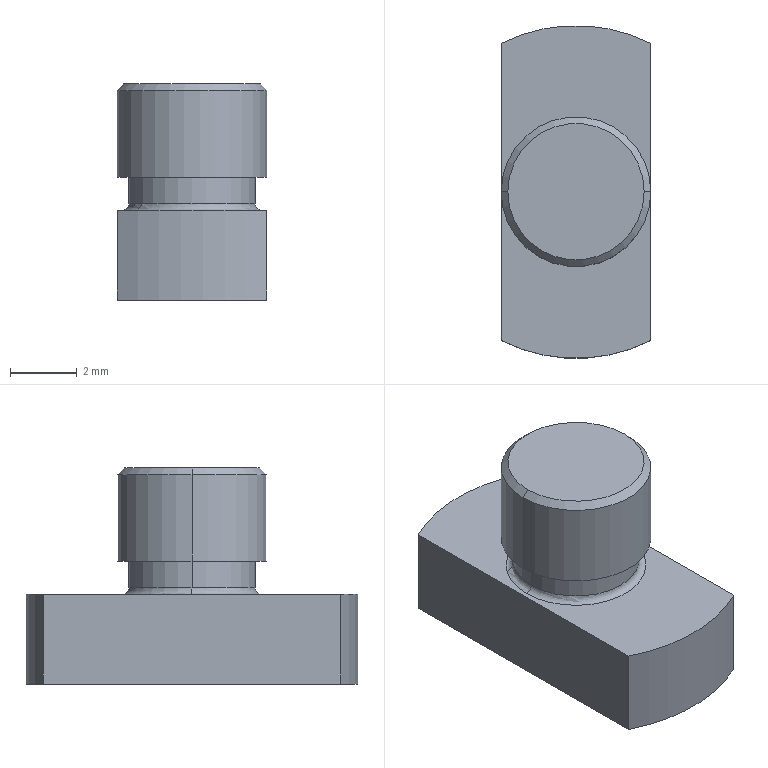Part | SolidWorks | features BaseBody 1 | 1 solid | 16 faces | box 4.5 x 10 x 6.5 mm | volume 172.969 mm3 | cylinder 6 | plane 6 | torus 2 | cone 2 | commonest cylinder face diameters 3.8 x2 4.5 x2 10 x2
STEP:
#1=CARTESIAN_POINT('',(76.4,38.,-17.3));
#2=VERTEX_POINT('',#1);
#3=CARTESIAN_POINT('',(72.6,38.,-17.3));
#4=VERTEX_POINT('',#3);
#5=CARTESIAN_POINT('',(74.5,38.,-17.3));
#6=DIRECTION('',(0.,0.,1.));
#7=DIRECTION('',(-1.,0.,0.));
#8=AXIS2_PLACEMENT_3D('',#5,#6,#7);
#9=CIRCLE('',#8,1.9);
#10=EDGE_CURVE('',#2,#4,#9,.T.);
#11=ORIENTED_EDGE('',*,*,#10,.F.);
#12=CARTESIAN_POINT('',(76.6,38.,-17.5));
#13=VERTEX_POINT('',#12);
#14=CARTESIAN_POINT('',(76.6,38.,-17.3));
#15=DIRECTION('',(0.,-1.,0.));
#16=DIRECTION('',(1.,0.,0.));
#17=AXIS2_PLACEMENT_3D('',#14,#15,#16);
#18=CIRCLE('',#17,0.2);
#19=EDGE_CURVE('',#2,#13,#18,.T.);
#20=ORIENTED_EDGE('',*,*,#19,.T.);
#21=CARTESIAN_POINT('',(72.4,38.,-17.5));
#22=VERTEX_POINT('',#21);
#23=CARTESIAN_POINT('',(74.5,38.,-17.5));
#24=DIRECTION('',(0.,0.,-1.));
#25=DIRECTION('',(-1.,0.,0.));
#26=AXIS2_PLACEMENT_3D('',#23,#24,#25);
#27=CIRCLE('',#26,2.1);
#28=EDGE_CURVE('',#22,#13,#27,.T.);
#29=ORIENTED_EDGE('',*,*,#28,.F.);
#30=CARTESIAN_POINT('',(72.4,38.,-17.3));
#31=DIRECTION('',(0.,1.,0.));
#32=DIRECTION('',(-1.,0.,0.));
#33=AXIS2_PLACEMENT_3D('',#30,#31,#32);
#34=CIRCLE('',#33,0.2);
#35=EDGE_CURVE('',#4,#22,#34,.T.);
#36=ORIENTED_EDGE('',*,*,#35,.F.);
#37=EDGE_LOOP('',(#11,#20,#29,#36));
#38=FACE_OUTER_BOUND('',#37,.T.);
#39=CARTESIAN_POINT('',(74.5,38.,-17.3));
#40=DIRECTION('',(0.,0.,1.));
#41=DIRECTION('',(-1.,0.,0.));
#42=AXIS2_PLACEMENT_3D('',#39,#40,#41);
#43=TOROIDAL_SURFACE('',#42,2.1,0.2);
#44=ADVANCED_FACE('',(#38),#43,.F.);
#45=CARTESIAN_POINT('',(76.55,38.,-13.7));
#46=VERTEX_POINT('',#45);
#47=CARTESIAN_POINT('',(72.45,38.,-13.7));
#48=VERTEX_POINT('',#47);
#49=CARTESIAN_POINT('',(74.5,38.,-13.7));
#50=DIRECTION('',(0.,0.,-1.));
#51=DIRECTION('',(1.,0.,0.));
#52=AXIS2_PLACEMENT_3D('',#49,#50,#51);
#53=CIRCLE('',#52,2.05);
#54=EDGE_CURVE('',#46,#48,#53,.T.);
#55=ORIENTED_EDGE('',*,*,#54,.T.);
#56=CARTESIAN_POINT('',(72.25,38.,-13.9));
#57=VERTEX_POINT('',#56);
#58=CARTESIAN_POINT('',(72.25,38.,-13.9));
#59=DIRECTION('',(-0.7071,0.,-0.7071));
#60=VECTOR('',#59,1000.);
#61=LINE('',#58,#60);
#62=EDGE_CURVE('',#48,#57,#61,.T.);
#63=ORIENTED_EDGE('',*,*,#62,.T.);
#64=CARTESIAN_POINT('',(76.75,38.,-13.9));
#65=VERTEX_POINT('',#64);
#66=CARTESIAN_POINT('',(74.5,38.,-13.9));
#67=DIRECTION('',(0.,0.,-1.));
#68=DIRECTION('',(1.,0.,0.));
#69=AXIS2_PLACEMENT_3D('',#66,#67,#68);
#70=CIRCLE('',#69,2.25);
#71=EDGE_CURVE('',#65,#57,#70,.T.);
#72=ORIENTED_EDGE('',*,*,#71,.F.);
#73=CARTESIAN_POINT('',(76.75,38.,-13.9));
#74=DIRECTION('',(0.7071,0.,-0.7071));
#75=VECTOR('',#74,1000.);
#76=LINE('',#73,#75);
#77=EDGE_CURVE('',#46,#65,#76,.T.);
#78=ORIENTED_EDGE('',*,*,#77,.F.);
#79=EDGE_LOOP('',(#55,#63,#72,#78));
#80=FACE_OUTER_BOUND('',#79,.T.);
#81=CARTESIAN_POINT('',(74.5,38.,-13.9));
#82=DIRECTION('',(0.,0.,-1.));
#83=DIRECTION('',(1.,0.,0.));
#84=AXIS2_PLACEMENT_3D('',#81,#82,#83);
#85=CONICAL_SURFACE('',#84,2.25,0.7854);
#86=ADVANCED_FACE('',(#80),#85,.T.);
#87=ORIENTED_EDGE('',*,*,#71,.T.);
#88=CARTESIAN_POINT('',(72.25,38.,-16.5));
#89=VERTEX_POINT('',#88);
#90=CARTESIAN_POINT('',(72.25,38.,-20.2));
#91=DIRECTION('',(0.,0.,-1.));
#92=VECTOR('',#91,1000.);
#93=LINE('',#90,#92);
#94=EDGE_CURVE('',#57,#89,#93,.T.);
#95=ORIENTED_EDGE('',*,*,#94,.T.);
#96=CARTESIAN_POINT('',(76.75,38.,-16.5));
#97=VERTEX_POINT('',#96);
#98=CARTESIAN_POINT('',(74.5,38.,-16.5));
#99=DIRECTION('',(0.,0.,-1.));
#100=DIRECTION('',(1.,0.,0.));
#101=AXIS2_PLACEMENT_3D('',#98,#99,#100);
#102=CIRCLE('',#101,2.25);
#103=EDGE_CURVE('',#97,#89,#102,.T.);
#104=ORIENTED_EDGE('',*,*,#103,.F.);
#105=CARTESIAN_POINT('',(76.75,38.,-20.2));
#106=DIRECTION('',(0.,0.,-1.));
#107=VECTOR('',#106,1000.);
#108=LINE('',#105,#107);
#109=EDGE_CURVE('',#65,#97,#108,.T.);
#110=ORIENTED_EDGE('',*,*,#109,.F.);
#111=EDGE_LOOP('',(#87,#95,#104,#110));
#112=FACE_OUTER_BOUND('',#111,.T.);
#113=CARTESIAN_POINT('',(74.5,38.,-20.2));
#114=DIRECTION('',(0.,0.,-1.));
#115=DIRECTION('',(1.,0.,0.));
#116=AXIS2_PLACEMENT_3D('',#113,#114,#115);
#117=CYLINDRICAL_SURFACE('',#116,2.25);
#118=ADVANCED_FACE('',(#112),#117,.T.);
#119=CARTESIAN_POINT('',(76.4,38.,-16.5));
#120=VERTEX_POINT('',#119);
#121=CARTESIAN_POINT('',(72.6,38.,-16.5));
#122=VERTEX_POINT('',#121);
#123=CARTESIAN_POINT('',(74.5,38.,-16.5));
#124=DIRECTION('',(0.,0.,-1.));
#125=DIRECTION('',(1.,0.,0.));
#126=AXIS2_PLACEMENT_3D('',#123,#124,#125);
#127=CIRCLE('',#126,1.9);
#128=EDGE_CURVE('',#120,#122,#127,.T.);
#129=ORIENTED_EDGE('',*,*,#128,.T.);
#130=CARTESIAN_POINT('',(72.6,38.,-20.2));
#131=DIRECTION('',(0.,0.,-1.));
#132=VECTOR('',#131,1000.);
#133=LINE('',#130,#132);
#134=EDGE_CURVE('',#122,#4,#133,.T.);
#135=ORIENTED_EDGE('',*,*,#134,.T.);
#136=CARTESIAN_POINT('',(74.5,38.,-17.3));
#137=DIRECTION('',(0.,0.,1.));
#138=DIRECTION('',(-1.,0.,0.));
#139=AXIS2_PLACEMENT_3D('',#136,#137,#138);
#140=CIRCLE('',#139,1.9);
#141=EDGE_CURVE('',#4,#2,#140,.T.);
#142=ORIENTED_EDGE('',*,*,#141,.T.);
#143=CARTESIAN_POINT('',(76.4,38.,-20.2));
#144=DIRECTION('',(0.,0.,-1.));
#145=VECTOR('',#144,1000.);
#146=LINE('',#143,#145);
#147=EDGE_CURVE('',#120,#2,#146,.T.);
#148=ORIENTED_EDGE('',*,*,#147,.F.);
#149=EDGE_LOOP('',(#129,#135,#142,#148));
#150=FACE_OUTER_BOUND('',#149,.T.);
#151=CARTESIAN_POINT('',(74.5,38.,-20.2));
#152=DIRECTION('',(0.,0.,-1.));
#153=DIRECTION('',(1.,0.,0.));
#154=AXIS2_PLACEMENT_3D('',#151,#152,#153);
#155=CYLINDRICAL_SURFACE('',#154,1.9);
#156=ADVANCED_FACE('',(#150),#155,.T.);
#157=CARTESIAN_POINT('',(76.75,33.535,-17.5));
#158=VERTEX_POINT('',#157);
#159=CARTESIAN_POINT('',(76.75,33.535,-20.2));
#160=VERTEX_POINT('',#159);
#161=CARTESIAN_POINT('',(76.75,33.535,-20.2));
#162=DIRECTION('',(0.,0.,-1.));
#163=VECTOR('',#162,1000.);
#164=LINE('',#161,#163);
#165=EDGE_CURVE('',#158,#160,#164,.T.);
#166=ORIENTED_EDGE('',*,*,#165,.F.);
#167=CARTESIAN_POINT('',(72.25,33.535,-17.5));
#168=VERTEX_POINT('',#167);
#169=CARTESIAN_POINT('',(74.5,38.,-17.5));
#170=DIRECTION('',(0.,0.,-1.));
#171=DIRECTION('',(1.,0.,0.));
#172=AXIS2_PLACEMENT_3D('',#169,#170,#171);
#173=CIRCLE('',#172,5.);
#174=EDGE_CURVE('',#158,#168,#173,.T.);
#175=ORIENTED_EDGE('',*,*,#174,.T.);
#176=CARTESIAN_POINT('',(72.25,33.535,-20.2));
#177=VERTEX_POINT('',#176);
#178=CARTESIAN_POINT('',(72.25,33.535,-20.2));
#179=DIRECTION('',(0.,0.,1.));
#180=VECTOR('',#179,1000.);
#181=LINE('',#178,#180);
#182=EDGE_CURVE('',#177,#168,#181,.T.);
#183=ORIENTED_EDGE('',*,*,#182,.F.);
#184=CARTESIAN_POINT('',(74.5,38.,-20.2));
#185=DIRECTION('',(0.,0.,-1.));
#186=DIRECTION('',(1.,0.,0.));
#187=AXIS2_PLACEMENT_3D('',#184,#185,#186);
#188=CIRCLE('',#187,5.);
#189=EDGE_CURVE('',#160,#177,#188,.T.);
#190=ORIENTED_EDGE('',*,*,#189,.F.);
#191=EDGE_LOOP('',(#166,#175,#183,#190));
#192=FACE_OUTER_BOUND('',#191,.T.);
#193=CARTESIAN_POINT('',(74.5,38.,-20.2));
#194=DIRECTION('',(0.,0.,-1.));
#195=DIRECTION('',(1.,0.,0.));
#196=AXIS2_PLACEMENT_3D('',#193,#194,#195);
#197=CYLINDRICAL_SURFACE('',#196,5.);
#198=ADVANCED_FACE('',(#192),#197,.T.);
#199=CARTESIAN_POINT('',(76.75,42.465,-20.2));
#200=VERTEX_POINT('',#199);
#201=CARTESIAN_POINT('',(76.75,43.,-20.2));
#202=DIRECTION('',(0.,1.,0.));
#203=VECTOR('',#202,1000.);
#204=LINE('',#201,#203);
#205=EDGE_CURVE('',#160,#200,#204,.T.);
#206=ORIENTED_EDGE('',*,*,#205,.F.);
#207=ORIENTED_EDGE('',*,*,#189,.T.);
#208=CARTESIAN_POINT('',(72.25,42.465,-20.2));
#209=VERTEX_POINT('',#208);
#210=CARTESIAN_POINT('',(72.25,43.,-20.2));
#211=DIRECTION('',(0.,-1.,0.));
#212=VECTOR('',#211,1000.);
#213=LINE('',#210,#212);
#214=EDGE_CURVE('',#209,#177,#213,.T.);
#215=ORIENTED_EDGE('',*,*,#214,.F.);
#216=CARTESIAN_POINT('',(74.5,38.,-20.2));
#217=DIRECTION('',(0.,0.,-1.));
#218=DIRECTION('',(1.,0.,0.));
#219=AXIS2_PLACEMENT_3D('',#216,#217,#218);
#220=CIRCLE('',#219,5.);
#221=EDGE_CURVE('',#209,#200,#220,.T.);
#222=ORIENTED_EDGE('',*,*,#221,.T.);
#223=EDGE_LOOP('',(#206,#207,#215,#222));
#224=FACE_OUTER_BOUND('',#223,.T.);
#225=CARTESIAN_POINT('',(74.5,38.,-20.2));
#226=DIRECTION('',(0.,0.,-1.));
#227=DIRECTION('',(1.,0.,0.));
#228=AXIS2_PLACEMENT_3D('',#225,#226,#227);
#229=PLANE('',#228);
#230=ADVANCED_FACE('',(#224),#229,.T.);
#231=CARTESIAN_POINT('',(72.25,42.465,-17.5));
#232=VERTEX_POINT('',#231);
#233=CARTESIAN_POINT('',(72.25,42.465,-20.2));
#234=DIRECTION('',(0.,0.,-1.));
#235=VECTOR('',#234,1000.);
#236=LINE('',#233,#235);
#237=EDGE_CURVE('',#232,#209,#236,.T.);
#238=ORIENTED_EDGE('',*,*,#237,.F.);
#239=CARTESIAN_POINT('',(76.75,42.465,-17.5));
#240=VERTEX_POINT('',#239);
#241=CARTESIAN_POINT('',(74.5,38.,-17.5));
#242=DIRECTION('',(0.,0.,-1.));
#243=DIRECTION('',(1.,0.,0.));
#244=AXIS2_PLACEMENT_3D('',#241,#242,#243);
#245=CIRCLE('',#244,5.);
#246=EDGE_CURVE('',#232,#240,#245,.T.);
#247=ORIENTED_EDGE('',*,*,#246,.T.);
#248=CARTESIAN_POINT('',(76.75,42.465,-20.2));
#249=DIRECTION('',(0.,0.,1.));
#250=VECTOR('',#249,1000.);
#251=LINE('',#248,#250);
#252=EDGE_CURVE('',#200,#240,#251,.T.);
#253=ORIENTED_EDGE('',*,*,#252,.F.);
#254=ORIENTED_EDGE('',*,*,#221,.F.);
#255=EDGE_LOOP('',(#238,#247,#253,#254));
#256=FACE_OUTER_BOUND('',#255,.T.);
#257=CARTESIAN_POINT('',(74.5,38.,-20.2));
#258=DIRECTION('',(0.,0.,-1.));
#259=DIRECTION('',(1.,0.,0.));
#260=AXIS2_PLACEMENT_3D('',#257,#258,#259);
#261=CYLINDRICAL_SURFACE('',#260,5.);
#262=ADVANCED_FACE('',(#256),#261,.T.);
#263=CARTESIAN_POINT('',(76.75,33.,-17.5));
#264=DIRECTION('',(0.,-1.,0.));
#265=VECTOR('',#264,1000.);
#266=LINE('',#263,#265);
#267=EDGE_CURVE('',#240,#158,#266,.T.);
#268=ORIENTED_EDGE('',*,*,#267,.F.);
#269=ORIENTED_EDGE('',*,*,#246,.F.);
#270=CARTESIAN_POINT('',(72.25,33.,-17.5));
#271=DIRECTION('',(0.,1.,0.));
#272=VECTOR('',#271,1000.);
#273=LINE('',#270,#272);
#274=EDGE_CURVE('',#168,#232,#273,.T.);
#275=ORIENTED_EDGE('',*,*,#274,.F.);
#276=ORIENTED_EDGE('',*,*,#174,.F.);
#277=EDGE_LOOP('',(#268,#269,#275,#276));
#278=FACE_OUTER_BOUND('',#277,.T.);
#279=ORIENTED_EDGE('',*,*,#28,.T.);
#280=CARTESIAN_POINT('',(74.5,38.,-17.5));
#281=DIRECTION('',(0.,0.,-1.));
#282=DIRECTION('',(-1.,0.,0.));
#283=AXIS2_PLACEMENT_3D('',#280,#281,#282);
#284=CIRCLE('',#283,2.1);
#285=EDGE_CURVE('',#13,#22,#284,.T.);
#286=ORIENTED_EDGE('',*,*,#285,.T.);
#287=EDGE_LOOP('',(#279,#286));
#288=FACE_BOUND('',#287,.T.);
#289=CARTESIAN_POINT('',(74.5,33.,-17.5));
#290=DIRECTION('',(0.,0.,1.));
#291=DIRECTION('',(-1.,0.,0.));
#292=AXIS2_PLACEMENT_3D('',#289,#290,#291);
#293=PLANE('',#292);
#294=ADVANCED_FACE('',(#278,#288),#293,.T.);
#295=ORIENTED_EDGE('',*,*,#134,.F.);
#296=CARTESIAN_POINT('',(74.5,38.,-16.5));
#297=DIRECTION('',(0.,0.,-1.));
#298=DIRECTION('',(1.,0.,0.));
#299=AXIS2_PLACEMENT_3D('',#296,#297,#298);
#300=CIRCLE('',#299,1.9);
#301=EDGE_CURVE('',#122,#120,#300,.T.);
#302=ORIENTED_EDGE('',*,*,#301,.T.);
#303=ORIENTED_EDGE('',*,*,#147,.T.);
#304=ORIENTED_EDGE('',*,*,#10,.T.);
#305=EDGE_LOOP('',(#295,#302,#303,#304));
#306=FACE_OUTER_BOUND('',#305,.T.);
#307=CARTESIAN_POINT('',(74.5,38.,-20.2));
#308=DIRECTION('',(0.,0.,-1.));
#309=DIRECTION('',(1.,0.,0.));
#310=AXIS2_PLACEMENT_3D('',#307,#308,#309);
#311=CYLINDRICAL_SURFACE('',#310,1.9);
#312=ADVANCED_FACE('',(#306),#311,.T.);
#313=ORIENTED_EDGE('',*,*,#103,.T.);
#314=CARTESIAN_POINT('',(74.5,38.,-16.5));
#315=DIRECTION('',(0.,0.,-1.));
#316=DIRECTION('',(1.,0.,0.));
#317=AXIS2_PLACEMENT_3D('',#314,#315,#316);
#318=CIRCLE('',#317,2.25);
#319=EDGE_CURVE('',#89,#97,#318,.T.);
#320=ORIENTED_EDGE('',*,*,#319,.T.);
#321=EDGE_LOOP('',(#313,#320));
#322=FACE_OUTER_BOUND('',#321,.T.);
#323=ORIENTED_EDGE('',*,*,#128,.F.);
#324=ORIENTED_EDGE('',*,*,#301,.F.);
#325=EDGE_LOOP('',(#323,#324));
#326=FACE_BOUND('',#325,.T.);
#327=CARTESIAN_POINT('',(74.5,36.1,-16.5));
#328=DIRECTION('',(0.,0.,-1.));
#329=DIRECTION('',(1.,0.,0.));
#330=AXIS2_PLACEMENT_3D('',#327,#328,#329);
#331=PLANE('',#330);
#332=ADVANCED_FACE('',(#322,#326),#331,.T.);
#333=ORIENTED_EDGE('',*,*,#94,.F.);
#334=CARTESIAN_POINT('',(74.5,38.,-13.9));
#335=DIRECTION('',(0.,0.,-1.));
#336=DIRECTION('',(1.,0.,0.));
#337=AXIS2_PLACEMENT_3D('',#334,#335,#336);
#338=CIRCLE('',#337,2.25);
#339=EDGE_CURVE('',#57,#65,#338,.T.);
#340=ORIENTED_EDGE('',*,*,#339,.T.);
#341=ORIENTED_EDGE('',*,*,#109,.T.);
#342=ORIENTED_EDGE('',*,*,#319,.F.);
#343=EDGE_LOOP('',(#333,#340,#341,#342));
#344=FACE_OUTER_BOUND('',#343,.T.);
#345=CARTESIAN_POINT('',(74.5,38.,-20.2));
#346=DIRECTION('',(0.,0.,-1.));
#347=DIRECTION('',(1.,0.,0.));
#348=AXIS2_PLACEMENT_3D('',#345,#346,#347);
#349=CYLINDRICAL_SURFACE('',#348,2.25);
#350=ADVANCED_FACE('',(#344),#349,.T.);
#351=ORIENTED_EDGE('',*,*,#62,.F.);
#352=CARTESIAN_POINT('',(74.5,38.,-13.7));
#353=DIRECTION('',(0.,0.,-1.));
#354=DIRECTION('',(1.,0.,0.));
#355=AXIS2_PLACEMENT_3D('',#352,#353,#354);
#356=CIRCLE('',#355,2.05);
#357=EDGE_CURVE('',#48,#46,#356,.T.);
#358=ORIENTED_EDGE('',*,*,#357,.T.);
#359=ORIENTED_EDGE('',*,*,#77,.T.);
#360=ORIENTED_EDGE('',*,*,#339,.F.);
#361=EDGE_LOOP('',(#351,#358,#359,#360));
#362=FACE_OUTER_BOUND('',#361,.T.);
#363=CARTESIAN_POINT('',(74.5,38.,-13.9));
#364=DIRECTION('',(0.,0.,-1.));
#365=DIRECTION('',(1.,0.,0.));
#366=AXIS2_PLACEMENT_3D('',#363,#364,#365);
#367=CONICAL_SURFACE('',#366,2.25,0.7854);
#368=ADVANCED_FACE('',(#362),#367,.T.);
#369=ORIENTED_EDGE('',*,*,#54,.F.);
#370=ORIENTED_EDGE('',*,*,#357,.F.);
#371=EDGE_LOOP('',(#369,#370));
#372=FACE_OUTER_BOUND('',#371,.T.);
#373=CARTESIAN_POINT('',(74.5,35.95,-13.7));
#374=DIRECTION('',(0.,0.,1.));
#375=DIRECTION('',(-1.,0.,0.));
#376=AXIS2_PLACEMENT_3D('',#373,#374,#375);
#377=PLANE('',#376);
#378=ADVANCED_FACE('',(#372),#377,.T.);
#379=ORIENTED_EDGE('',*,*,#19,.F.);
#380=ORIENTED_EDGE('',*,*,#141,.F.);
#381=ORIENTED_EDGE('',*,*,#35,.T.);
#382=ORIENTED_EDGE('',*,*,#285,.F.);
#383=EDGE_LOOP('',(#379,#380,#381,#382));
#384=FACE_OUTER_BOUND('',#383,.T.);
#385=CARTESIAN_POINT('',(74.5,38.,-17.3));
#386=DIRECTION('',(0.,0.,1.));
#387=DIRECTION('',(-1.,0.,0.));
#388=AXIS2_PLACEMENT_3D('',#385,#386,#387);
#389=TOROIDAL_SURFACE('',#388,2.1,0.2);
#390=ADVANCED_FACE('',(#384),#389,.F.);
#391=ORIENTED_EDGE('',*,*,#182,.T.);
#392=ORIENTED_EDGE('',*,*,#274,.T.);
#393=ORIENTED_EDGE('',*,*,#237,.T.);
#394=ORIENTED_EDGE('',*,*,#214,.T.);
#395=EDGE_LOOP('',(#391,#392,#393,#394));
#396=FACE_OUTER_BOUND('',#395,.T.);
#397=CARTESIAN_POINT('',(72.25,43.,-2.595));
#398=DIRECTION('',(1.,0.,0.));
#399=DIRECTION('',(0.,1.,0.));
#400=AXIS2_PLACEMENT_3D('',#397,#398,#399);
#401=PLANE('',#400);
#402=ADVANCED_FACE('',(#396),#401,.F.);
#403=ORIENTED_EDGE('',*,*,#252,.T.);
#404=ORIENTED_EDGE('',*,*,#267,.T.);
#405=ORIENTED_EDGE('',*,*,#165,.T.);
#406=ORIENTED_EDGE('',*,*,#205,.T.);
#407=EDGE_LOOP('',(#403,#404,#405,#406));
#408=FACE_OUTER_BOUND('',#407,.T.);
#409=CARTESIAN_POINT('',(76.75,43.,-2.595));
#410=DIRECTION('',(-1.,0.,0.));
#411=DIRECTION('',(0.,-1.,0.));
#412=AXIS2_PLACEMENT_3D('',#409,#410,#411);
#413=PLANE('',#412);
#414=ADVANCED_FACE('',(#408),#413,.F.);
#415=CLOSED_SHELL('',(#44,#86,#118,#156,#198,#230,#262,#294,#312,#332,#350,#368,#378,#390,#402,#414));
#416=MANIFOLD_SOLID_BREP('',#415);
#417=CARTESIAN_POINT('',(0.,0.,0.));
#418=DIRECTION('',(0.,0.,1.));
#419=DIRECTION('',(1.,0.,0.));
#420=AXIS2_PLACEMENT_3D('',#417,#418,#419);
#421=(LENGTH_UNIT()NAMED_UNIT(*)SI_UNIT(.MILLI.,.METRE.));
#422=UNCERTAINTY_MEASURE_WITH_UNIT(LENGTH_MEASURE(0.00001),#421,'','');
#423=(NAMED_UNIT(*)PLANE_ANGLE_UNIT()SI_UNIT($,.RADIAN.));
#424=(NAMED_UNIT(*)SI_UNIT($,.STERADIAN.)SOLID_ANGLE_UNIT());
#425=(GEOMETRIC_REPRESENTATION_CONTEXT(3)GLOBAL_UNCERTAINTY_ASSIGNED_CONTEXT((#422))GLOBAL_UNIT_ASSIGNED_CONTEXT((#421,#423,#424))REPRESENTATION_CONTEXT('',''));
#426=ADVANCED_BREP_SHAPE_REPRESENTATION('',(#416,#420),#425);